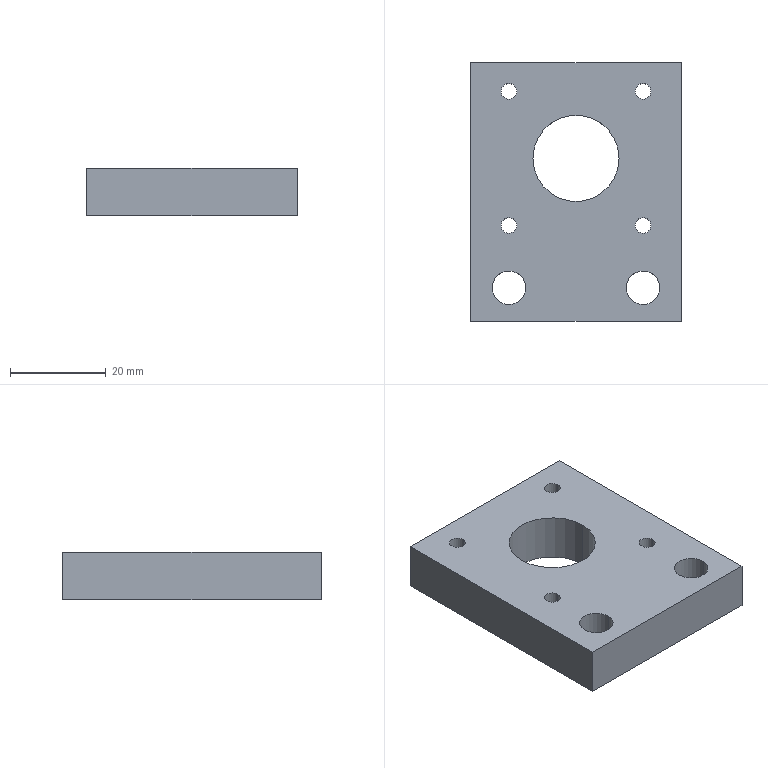Part | NX | 1 solid | 28 faces | box 44 x 54 x 10 mm | volume 20097 mm3 | cylinder 14 | cone 8 | plane 6 | commonest cylinder face diameters 3.3 x8 7 x4 18 x2
STEP:
#1=CARTESIAN_POINT('',(566.5,55.4,-338.82));
#2=VERTEX_POINT('',#1);
#3=CARTESIAN_POINT('',(573.5,55.4,-338.82));
#4=VERTEX_POINT('',#3);
#5=CARTESIAN_POINT('',(570.,55.4,-338.82));
#6=DIRECTION('',(0.,0.,1.));
#7=DIRECTION('',(1.,0.,0.));
#8=AXIS2_PLACEMENT_3D('',#5,#6,#7);
#9=CIRCLE('',#8,3.5);
#10=EDGE_CURVE('',#2,#4,#9,.T.);
#11=ORIENTED_EDGE('',*,*,#10,.F.);
#12=CARTESIAN_POINT('',(566.5,55.4,-328.82));
#13=VERTEX_POINT('',#12);
#14=CARTESIAN_POINT('',(566.5,55.4,-338.82));
#15=DIRECTION('',(0.,0.,1.));
#16=VECTOR('',#15,1000.);
#17=LINE('',#14,#16);
#18=EDGE_CURVE('',#2,#13,#17,.T.);
#19=ORIENTED_EDGE('',*,*,#18,.T.);
#20=CARTESIAN_POINT('',(573.5,55.4,-328.82));
#21=VERTEX_POINT('',#20);
#22=CARTESIAN_POINT('',(570.,55.4,-328.82));
#23=DIRECTION('',(0.,0.,1.));
#24=DIRECTION('',(1.,0.,0.));
#25=AXIS2_PLACEMENT_3D('',#22,#23,#24);
#26=CIRCLE('',#25,3.5);
#27=EDGE_CURVE('',#13,#21,#26,.T.);
#28=ORIENTED_EDGE('',*,*,#27,.T.);
#29=CARTESIAN_POINT('',(573.5,55.4,-338.82));
#30=DIRECTION('',(0.,0.,1.));
#31=VECTOR('',#30,1000.);
#32=LINE('',#29,#31);
#33=EDGE_CURVE('',#4,#21,#32,.T.);
#34=ORIENTED_EDGE('',*,*,#33,.F.);
#35=EDGE_LOOP('',(#11,#19,#28,#34));
#36=FACE_BOUND('',#35,.T.);
#37=CARTESIAN_POINT('',(570.,55.4,-338.82));
#38=DIRECTION('',(0.,0.,1.));
#39=DIRECTION('',(1.,0.,0.));
#40=AXIS2_PLACEMENT_3D('',#37,#38,#39);
#41=CYLINDRICAL_SURFACE('',#40,3.5);
#42=ADVANCED_FACE('',(#36),#41,.F.);
#43=CARTESIAN_POINT('',(578.,102.4,-338.82));
#44=VERTEX_POINT('',#43);
#45=CARTESIAN_POINT('',(578.,48.4,-338.82));
#46=VERTEX_POINT('',#45);
#47=CARTESIAN_POINT('',(578.,0.,-338.82));
#48=DIRECTION('',(0.,-1.,0.));
#49=VECTOR('',#48,1000.);
#50=LINE('',#47,#49);
#51=EDGE_CURVE('',#44,#46,#50,.T.);
#52=ORIENTED_EDGE('',*,*,#51,.F.);
#53=CARTESIAN_POINT('',(578.,102.4,-328.82));
#54=VERTEX_POINT('',#53);
#55=CARTESIAN_POINT('',(578.,102.4,-338.82));
#56=DIRECTION('',(0.,0.,1.));
#57=VECTOR('',#56,1000.);
#58=LINE('',#55,#57);
#59=EDGE_CURVE('',#44,#54,#58,.T.);
#60=ORIENTED_EDGE('',*,*,#59,.T.);
#61=CARTESIAN_POINT('',(578.,48.4,-328.82));
#62=VERTEX_POINT('',#61);
#63=CARTESIAN_POINT('',(578.,0.,-328.82));
#64=DIRECTION('',(0.,-1.,0.));
#65=VECTOR('',#64,1000.);
#66=LINE('',#63,#65);
#67=EDGE_CURVE('',#54,#62,#66,.T.);
#68=ORIENTED_EDGE('',*,*,#67,.T.);
#69=CARTESIAN_POINT('',(578.,48.4,-338.82));
#70=DIRECTION('',(0.,0.,1.));
#71=VECTOR('',#70,1000.);
#72=LINE('',#69,#71);
#73=EDGE_CURVE('',#46,#62,#72,.T.);
#74=ORIENTED_EDGE('',*,*,#73,.F.);
#75=EDGE_LOOP('',(#52,#60,#68,#74));
#76=FACE_BOUND('',#75,.T.);
#77=CARTESIAN_POINT('',(578.,102.4,-338.82));
#78=DIRECTION('',(1.,0.,0.));
#79=DIRECTION('',(0.,1.,0.));
#80=AXIS2_PLACEMENT_3D('',#77,#78,#79);
#81=PLANE('',#80);
#82=ADVANCED_FACE('',(#76),#81,.T.);
#83=CARTESIAN_POINT('',(534.,48.4,-338.82));
#84=VERTEX_POINT('',#83);
#85=CARTESIAN_POINT('',(0.,48.4,-338.82));
#86=DIRECTION('',(-1.,0.,0.));
#87=VECTOR('',#86,1000.);
#88=LINE('',#85,#87);
#89=EDGE_CURVE('',#46,#84,#88,.T.);
#90=ORIENTED_EDGE('',*,*,#89,.F.);
#91=ORIENTED_EDGE('',*,*,#73,.T.);
#92=CARTESIAN_POINT('',(534.,48.4,-328.82));
#93=VERTEX_POINT('',#92);
#94=CARTESIAN_POINT('',(0.,48.4,-328.82));
#95=DIRECTION('',(-1.,0.,0.));
#96=VECTOR('',#95,1000.);
#97=LINE('',#94,#96);
#98=EDGE_CURVE('',#62,#93,#97,.T.);
#99=ORIENTED_EDGE('',*,*,#98,.T.);
#100=CARTESIAN_POINT('',(534.,48.4,-338.82));
#101=DIRECTION('',(0.,0.,1.));
#102=VECTOR('',#101,1000.);
#103=LINE('',#100,#102);
#104=EDGE_CURVE('',#84,#93,#103,.T.);
#105=ORIENTED_EDGE('',*,*,#104,.F.);
#106=EDGE_LOOP('',(#90,#91,#99,#105));
#107=FACE_BOUND('',#106,.T.);
#108=CARTESIAN_POINT('',(578.,48.4,-338.82));
#109=DIRECTION('',(0.,-1.,0.));
#110=DIRECTION('',(0.,0.,-1.));
#111=AXIS2_PLACEMENT_3D('',#108,#109,#110);
#112=PLANE('',#111);
#113=ADVANCED_FACE('',(#107),#112,.T.);
#114=CARTESIAN_POINT('',(534.,102.4,-338.82));
#115=VERTEX_POINT('',#114);
#116=CARTESIAN_POINT('',(0.,102.4,-338.82));
#117=DIRECTION('',(1.,0.,0.));
#118=VECTOR('',#117,1000.);
#119=LINE('',#116,#118);
#120=EDGE_CURVE('',#115,#44,#119,.T.);
#121=ORIENTED_EDGE('',*,*,#120,.F.);
#122=CARTESIAN_POINT('',(534.,102.4,-328.82));
#123=VERTEX_POINT('',#122);
#124=CARTESIAN_POINT('',(534.,102.4,-338.82));
#125=DIRECTION('',(0.,0.,1.));
#126=VECTOR('',#125,1000.);
#127=LINE('',#124,#126);
#128=EDGE_CURVE('',#115,#123,#127,.T.);
#129=ORIENTED_EDGE('',*,*,#128,.T.);
#130=CARTESIAN_POINT('',(0.,102.4,-328.82));
#131=DIRECTION('',(1.,0.,0.));
#132=VECTOR('',#131,1000.);
#133=LINE('',#130,#132);
#134=EDGE_CURVE('',#123,#54,#133,.T.);
#135=ORIENTED_EDGE('',*,*,#134,.T.);
#136=ORIENTED_EDGE('',*,*,#59,.F.);
#137=EDGE_LOOP('',(#121,#129,#135,#136));
#138=FACE_BOUND('',#137,.T.);
#139=CARTESIAN_POINT('',(534.,102.4,-338.82));
#140=DIRECTION('',(0.,1.,0.));
#141=DIRECTION('',(1.,0.,0.));
#142=AXIS2_PLACEMENT_3D('',#139,#140,#141);
#143=PLANE('',#142);
#144=ADVANCED_FACE('',(#138),#143,.T.);
#145=ORIENTED_EDGE('',*,*,#134,.F.);
#146=CARTESIAN_POINT('',(534.,0.,-328.82));
#147=DIRECTION('',(0.,1.,0.));
#148=VECTOR('',#147,1000.);
#149=LINE('',#146,#148);
#150=EDGE_CURVE('',#93,#123,#149,.T.);
#151=ORIENTED_EDGE('',*,*,#150,.F.);
#152=ORIENTED_EDGE('',*,*,#98,.F.);
#153=ORIENTED_EDGE('',*,*,#67,.F.);
#154=EDGE_LOOP('',(#145,#151,#152,#153));
#155=FACE_BOUND('',#154,.T.);
#156=CARTESIAN_POINT('',(545.5,55.4,-328.82));
#157=VERTEX_POINT('',#156);
#158=CARTESIAN_POINT('',(538.5,55.4,-328.82));
#159=VERTEX_POINT('',#158);
#160=CARTESIAN_POINT('',(542.,55.4,-328.82));
#161=DIRECTION('',(0.,0.,1.));
#162=DIRECTION('',(1.,0.,0.));
#163=AXIS2_PLACEMENT_3D('',#160,#161,#162);
#164=CIRCLE('',#163,3.5);
#165=EDGE_CURVE('',#157,#159,#164,.T.);
#166=ORIENTED_EDGE('',*,*,#165,.F.);
#167=CARTESIAN_POINT('',(542.,55.4,-328.82));
#168=DIRECTION('',(0.,0.,1.));
#169=DIRECTION('',(1.,0.,0.));
#170=AXIS2_PLACEMENT_3D('',#167,#168,#169);
#171=CIRCLE('',#170,3.5);
#172=EDGE_CURVE('',#159,#157,#171,.T.);
#173=ORIENTED_EDGE('',*,*,#172,.F.);
#174=EDGE_LOOP('',(#166,#173));
#175=FACE_BOUND('',#174,.T.);
#176=ORIENTED_EDGE('',*,*,#27,.F.);
#177=CARTESIAN_POINT('',(570.,55.4,-328.82));
#178=DIRECTION('',(0.,0.,1.));
#179=DIRECTION('',(1.,0.,0.));
#180=AXIS2_PLACEMENT_3D('',#177,#178,#179);
#181=CIRCLE('',#180,3.5);
#182=EDGE_CURVE('',#21,#13,#181,.T.);
#183=ORIENTED_EDGE('',*,*,#182,.F.);
#184=EDGE_LOOP('',(#176,#183));
#185=FACE_BOUND('',#184,.T.);
#186=CARTESIAN_POINT('',(547.,82.4,-328.82));
#187=VERTEX_POINT('',#186);
#188=CARTESIAN_POINT('',(565.,82.4,-328.82));
#189=VERTEX_POINT('',#188);
#190=CARTESIAN_POINT('',(556.,82.4,-328.82));
#191=DIRECTION('',(0.,0.,1.));
#192=DIRECTION('',(1.,0.,0.));
#193=AXIS2_PLACEMENT_3D('',#190,#191,#192);
#194=CIRCLE('',#193,9.);
#195=EDGE_CURVE('',#187,#189,#194,.T.);
#196=ORIENTED_EDGE('',*,*,#195,.F.);
#197=CARTESIAN_POINT('',(556.,82.4,-328.82));
#198=DIRECTION('',(0.,0.,1.));
#199=DIRECTION('',(1.,0.,0.));
#200=AXIS2_PLACEMENT_3D('',#197,#198,#199);
#201=CIRCLE('',#200,9.);
#202=EDGE_CURVE('',#189,#187,#201,.T.);
#203=ORIENTED_EDGE('',*,*,#202,.F.);
#204=EDGE_LOOP('',(#196,#203));
#205=FACE_BOUND('',#204,.T.);
#206=CARTESIAN_POINT('',(540.35,96.4,-328.82));
#207=VERTEX_POINT('',#206);
#208=CARTESIAN_POINT('',(543.65,96.4,-328.82));
#209=VERTEX_POINT('',#208);
#210=CARTESIAN_POINT('',(542.,96.4,-328.82));
#211=DIRECTION('',(0.,0.,-1.));
#212=DIRECTION('',(-1.,0.,0.));
#213=AXIS2_PLACEMENT_3D('',#210,#211,#212);
#214=CIRCLE('',#213,1.65);
#215=EDGE_CURVE('',#207,#209,#214,.T.);
#216=ORIENTED_EDGE('',*,*,#215,.T.);
#217=CARTESIAN_POINT('',(542.,96.4,-328.82));
#218=DIRECTION('',(0.,0.,-1.));
#219=DIRECTION('',(-1.,0.,0.));
#220=AXIS2_PLACEMENT_3D('',#217,#218,#219);
#221=CIRCLE('',#220,1.65);
#222=EDGE_CURVE('',#209,#207,#221,.T.);
#223=ORIENTED_EDGE('',*,*,#222,.T.);
#224=EDGE_LOOP('',(#216,#223));
#225=FACE_BOUND('',#224,.T.);
#226=CARTESIAN_POINT('',(540.35,68.4,-328.82));
#227=VERTEX_POINT('',#226);
#228=CARTESIAN_POINT('',(543.65,68.4,-328.82));
#229=VERTEX_POINT('',#228);
#230=CARTESIAN_POINT('',(542.,68.4,-328.82));
#231=DIRECTION('',(0.,0.,-1.));
#232=DIRECTION('',(-1.,0.,0.));
#233=AXIS2_PLACEMENT_3D('',#230,#231,#232);
#234=CIRCLE('',#233,1.65);
#235=EDGE_CURVE('',#227,#229,#234,.T.);
#236=ORIENTED_EDGE('',*,*,#235,.T.);
#237=CARTESIAN_POINT('',(542.,68.4,-328.82));
#238=DIRECTION('',(0.,0.,-1.));
#239=DIRECTION('',(-1.,0.,0.));
#240=AXIS2_PLACEMENT_3D('',#237,#238,#239);
#241=CIRCLE('',#240,1.65);
#242=EDGE_CURVE('',#229,#227,#241,.T.);
#243=ORIENTED_EDGE('',*,*,#242,.T.);
#244=EDGE_LOOP('',(#236,#243));
#245=FACE_BOUND('',#244,.T.);
#246=CARTESIAN_POINT('',(571.65,68.4,-328.82));
#247=VERTEX_POINT('',#246);
#248=CARTESIAN_POINT('',(568.35,68.4,-328.82));
#249=VERTEX_POINT('',#248);
#250=CARTESIAN_POINT('',(570.,68.4,-328.82));
#251=DIRECTION('',(0.,0.,-1.));
#252=DIRECTION('',(-1.,0.,0.));
#253=AXIS2_PLACEMENT_3D('',#250,#251,#252);
#254=CIRCLE('',#253,1.65);
#255=EDGE_CURVE('',#247,#249,#254,.T.);
#256=ORIENTED_EDGE('',*,*,#255,.T.);
#257=CARTESIAN_POINT('',(570.,68.4,-328.82));
#258=DIRECTION('',(0.,0.,-1.));
#259=DIRECTION('',(-1.,0.,0.));
#260=AXIS2_PLACEMENT_3D('',#257,#258,#259);
#261=CIRCLE('',#260,1.65);
#262=EDGE_CURVE('',#249,#247,#261,.T.);
#263=ORIENTED_EDGE('',*,*,#262,.T.);
#264=EDGE_LOOP('',(#256,#263));
#265=FACE_BOUND('',#264,.T.);
#266=CARTESIAN_POINT('',(568.35,96.4,-328.82));
#267=VERTEX_POINT('',#266);
#268=CARTESIAN_POINT('',(571.65,96.4,-328.82));
#269=VERTEX_POINT('',#268);
#270=CARTESIAN_POINT('',(570.,96.4,-328.82));
#271=DIRECTION('',(0.,0.,-1.));
#272=DIRECTION('',(-1.,0.,0.));
#273=AXIS2_PLACEMENT_3D('',#270,#271,#272);
#274=CIRCLE('',#273,1.65);
#275=EDGE_CURVE('',#267,#269,#274,.T.);
#276=ORIENTED_EDGE('',*,*,#275,.T.);
#277=CARTESIAN_POINT('',(570.,96.4,-328.82));
#278=DIRECTION('',(0.,0.,-1.));
#279=DIRECTION('',(-1.,0.,0.));
#280=AXIS2_PLACEMENT_3D('',#277,#278,#279);
#281=CIRCLE('',#280,1.65);
#282=EDGE_CURVE('',#269,#267,#281,.T.);
#283=ORIENTED_EDGE('',*,*,#282,.T.);
#284=EDGE_LOOP('',(#276,#283));
#285=FACE_BOUND('',#284,.T.);
#286=CARTESIAN_POINT('',(565.967,77.363,-328.82));
#287=DIRECTION('',(0.,0.,1.));
#288=DIRECTION('',(1.,0.,0.));
#289=AXIS2_PLACEMENT_3D('',#286,#287,#288);
#290=PLANE('',#289);
#291=ADVANCED_FACE('',(#155,#175,#185,#205,#225,#245,#265,#285),#290,.T.);
#292=ORIENTED_EDGE('',*,*,#195,.T.);
#293=CARTESIAN_POINT('',(565.,82.4,-338.82));
#294=VERTEX_POINT('',#293);
#295=CARTESIAN_POINT('',(565.,82.4,-339.82));
#296=DIRECTION('',(0.,0.,1.));
#297=VECTOR('',#296,1000.);
#298=LINE('',#295,#297);
#299=EDGE_CURVE('',#294,#189,#298,.T.);
#300=ORIENTED_EDGE('',*,*,#299,.F.);
#301=CARTESIAN_POINT('',(547.,82.4,-338.82));
#302=VERTEX_POINT('',#301);
#303=CARTESIAN_POINT('',(556.,82.4,-338.82));
#304=DIRECTION('',(0.,0.,1.));
#305=DIRECTION('',(1.,0.,0.));
#306=AXIS2_PLACEMENT_3D('',#303,#304,#305);
#307=CIRCLE('',#306,9.);
#308=EDGE_CURVE('',#302,#294,#307,.T.);
#309=ORIENTED_EDGE('',*,*,#308,.F.);
#310=CARTESIAN_POINT('',(547.,82.4,-339.82));
#311=DIRECTION('',(0.,0.,1.));
#312=VECTOR('',#311,1000.);
#313=LINE('',#310,#312);
#314=EDGE_CURVE('',#302,#187,#313,.T.);
#315=ORIENTED_EDGE('',*,*,#314,.T.);
#316=EDGE_LOOP('',(#292,#300,#309,#315));
#317=FACE_BOUND('',#316,.T.);
#318=CARTESIAN_POINT('',(556.,82.4,-339.82));
#319=DIRECTION('',(0.,0.,1.));
#320=DIRECTION('',(1.,0.,0.));
#321=AXIS2_PLACEMENT_3D('',#318,#319,#320);
#322=CYLINDRICAL_SURFACE('',#321,9.);
#323=ADVANCED_FACE('',(#317),#322,.F.);
#324=CARTESIAN_POINT('',(534.,0.,-338.82));
#325=DIRECTION('',(0.,1.,0.));
#326=VECTOR('',#325,1000.);
#327=LINE('',#324,#326);
#328=EDGE_CURVE('',#84,#115,#327,.T.);
#329=ORIENTED_EDGE('',*,*,#328,.F.);
#330=ORIENTED_EDGE('',*,*,#104,.T.);
#331=ORIENTED_EDGE('',*,*,#150,.T.);
#332=ORIENTED_EDGE('',*,*,#128,.F.);
#333=EDGE_LOOP('',(#329,#330,#331,#332));
#334=FACE_BOUND('',#333,.T.);
#335=CARTESIAN_POINT('',(534.,48.4,-338.82));
#336=DIRECTION('',(-1.,0.,0.));
#337=DIRECTION('',(0.,0.,1.));
#338=AXIS2_PLACEMENT_3D('',#335,#336,#337);
#339=PLANE('',#338);
#340=ADVANCED_FACE('',(#334),#339,.T.);
#341=CARTESIAN_POINT('',(545.5,55.4,-338.82));
#342=VERTEX_POINT('',#341);
#343=CARTESIAN_POINT('',(538.5,55.4,-338.82));
#344=VERTEX_POINT('',#343);
#345=CARTESIAN_POINT('',(542.,55.4,-338.82));
#346=DIRECTION('',(0.,0.,1.));
#347=DIRECTION('',(1.,0.,0.));
#348=AXIS2_PLACEMENT_3D('',#345,#346,#347);
#349=CIRCLE('',#348,3.5);
#350=EDGE_CURVE('',#342,#344,#349,.T.);
#351=ORIENTED_EDGE('',*,*,#350,.F.);
#352=CARTESIAN_POINT('',(545.5,55.4,-338.82));
#353=DIRECTION('',(0.,0.,1.));
#354=VECTOR('',#353,1000.);
#355=LINE('',#352,#354);
#356=EDGE_CURVE('',#342,#157,#355,.T.);
#357=ORIENTED_EDGE('',*,*,#356,.T.);
#358=ORIENTED_EDGE('',*,*,#165,.T.);
#359=CARTESIAN_POINT('',(538.5,55.4,-338.82));
#360=DIRECTION('',(0.,0.,1.));
#361=VECTOR('',#360,1000.);
#362=LINE('',#359,#361);
#363=EDGE_CURVE('',#344,#159,#362,.T.);
#364=ORIENTED_EDGE('',*,*,#363,.F.);
#365=EDGE_LOOP('',(#351,#357,#358,#364));
#366=FACE_BOUND('',#365,.T.);
#367=CARTESIAN_POINT('',(542.,55.4,-338.82));
#368=DIRECTION('',(0.,0.,1.));
#369=DIRECTION('',(1.,0.,0.));
#370=AXIS2_PLACEMENT_3D('',#367,#368,#369);
#371=CYLINDRICAL_SURFACE('',#370,3.5);
#372=ADVANCED_FACE('',(#366),#371,.F.);
#373=ORIENTED_EDGE('',*,*,#51,.T.);
#374=ORIENTED_EDGE('',*,*,#89,.T.);
#375=ORIENTED_EDGE('',*,*,#328,.T.);
#376=ORIENTED_EDGE('',*,*,#120,.T.);
#377=EDGE_LOOP('',(#373,#374,#375,#376));
#378=FACE_BOUND('',#377,.T.);
#379=ORIENTED_EDGE('',*,*,#350,.T.);
#380=CARTESIAN_POINT('',(542.,55.4,-338.82));
#381=DIRECTION('',(0.,0.,1.));
#382=DIRECTION('',(1.,0.,0.));
#383=AXIS2_PLACEMENT_3D('',#380,#381,#382);
#384=CIRCLE('',#383,3.5);
#385=EDGE_CURVE('',#344,#342,#384,.T.);
#386=ORIENTED_EDGE('',*,*,#385,.T.);
#387=EDGE_LOOP('',(#379,#386));
#388=FACE_BOUND('',#387,.T.);
#389=CARTESIAN_POINT('',(572.315,96.4,-338.82));
#390=VERTEX_POINT('',#389);
#391=CARTESIAN_POINT('',(567.685,96.4,-338.82));
#392=VERTEX_POINT('',#391);
#393=CARTESIAN_POINT('',(570.,96.4,-338.82));
#394=DIRECTION('',(0.,0.,-1.));
#395=DIRECTION('',(-1.,0.,0.));
#396=AXIS2_PLACEMENT_3D('',#393,#394,#395);
#397=CIRCLE('',#396,2.315);
#398=EDGE_CURVE('',#390,#392,#397,.T.);
#399=ORIENTED_EDGE('',*,*,#398,.F.);
#400=CARTESIAN_POINT('',(570.,96.4,-338.82));
#401=DIRECTION('',(0.,0.,-1.));
#402=DIRECTION('',(-1.,0.,0.));
#403=AXIS2_PLACEMENT_3D('',#400,#401,#402);
#404=CIRCLE('',#403,2.315);
#405=EDGE_CURVE('',#392,#390,#404,.T.);
#406=ORIENTED_EDGE('',*,*,#405,.F.);
#407=EDGE_LOOP('',(#399,#406));
#408=FACE_BOUND('',#407,.T.);
#409=CARTESIAN_POINT('',(544.315,68.4,-338.82));
#410=VERTEX_POINT('',#409);
#411=CARTESIAN_POINT('',(539.685,68.4,-338.82));
#412=VERTEX_POINT('',#411);
#413=CARTESIAN_POINT('',(542.,68.4,-338.82));
#414=DIRECTION('',(0.,0.,-1.));
#415=DIRECTION('',(-1.,0.,0.));
#416=AXIS2_PLACEMENT_3D('',#413,#414,#415);
#417=CIRCLE('',#416,2.315);
#418=EDGE_CURVE('',#410,#412,#417,.T.);
#419=ORIENTED_EDGE('',*,*,#418,.F.);
#420=CARTESIAN_POINT('',(542.,68.4,-338.82));
#421=DIRECTION('',(0.,0.,-1.));
#422=DIRECTION('',(-1.,0.,0.));
#423=AXIS2_PLACEMENT_3D('',#420,#421,#422);
#424=CIRCLE('',#423,2.315);
#425=EDGE_CURVE('',#412,#410,#424,.T.);
#426=ORIENTED_EDGE('',*,*,#425,.F.);
#427=EDGE_LOOP('',(#419,#426));
#428=FACE_BOUND('',#427,.T.);
#429=ORIENTED_EDGE('',*,*,#10,.T.);
#430=CARTESIAN_POINT('',(570.,55.4,-338.82));
#431=DIRECTION('',(0.,0.,1.));
#432=DIRECTION('',(1.,0.,0.));
#433=AXIS2_PLACEMENT_3D('',#430,#431,#432);
#434=CIRCLE('',#433,3.5);
#435=EDGE_CURVE('',#4,#2,#434,.T.);
#436=ORIENTED_EDGE('',*,*,#435,.T.);
#437=EDGE_LOOP('',(#429,#436));
#438=FACE_BOUND('',#437,.T.);
#439=CARTESIAN_POINT('',(556.,82.4,-338.82));
#440=DIRECTION('',(0.,0.,1.));
#441=DIRECTION('',(1.,0.,0.));
#442=AXIS2_PLACEMENT_3D('',#439,#440,#441);
#443=CIRCLE('',#442,9.);
#444=EDGE_CURVE('',#294,#302,#443,.T.);
#445=ORIENTED_EDGE('',*,*,#444,.T.);
#446=ORIENTED_EDGE('',*,*,#308,.T.);
#447=EDGE_LOOP('',(#445,#446));
#448=FACE_BOUND('',#447,.T.);
#449=CARTESIAN_POINT('',(539.685,96.4,-338.82));
#450=VERTEX_POINT('',#449);
#451=CARTESIAN_POINT('',(544.315,96.4,-338.82));
#452=VERTEX_POINT('',#451);
#453=CARTESIAN_POINT('',(542.,96.4,-338.82));
#454=DIRECTION('',(0.,0.,-1.));
#455=DIRECTION('',(-1.,0.,0.));
#456=AXIS2_PLACEMENT_3D('',#453,#454,#455);
#457=CIRCLE('',#456,2.315);
#458=EDGE_CURVE('',#450,#452,#457,.T.);
#459=ORIENTED_EDGE('',*,*,#458,.F.);
#460=CARTESIAN_POINT('',(542.,96.4,-338.82));
#461=DIRECTION('',(0.,0.,-1.));
#462=DIRECTION('',(-1.,0.,0.));
#463=AXIS2_PLACEMENT_3D('',#460,#461,#462);
#464=CIRCLE('',#463,2.315);
#465=EDGE_CURVE('',#452,#450,#464,.T.);
#466=ORIENTED_EDGE('',*,*,#465,.F.);
#467=EDGE_LOOP('',(#459,#466));
#468=FACE_BOUND('',#467,.T.);
#469=CARTESIAN_POINT('',(567.685,68.4,-338.82));
#470=VERTEX_POINT('',#469);
#471=CARTESIAN_POINT('',(572.315,68.4,-338.82));
#472=VERTEX_POINT('',#471);
#473=CARTESIAN_POINT('',(570.,68.4,-338.82));
#474=DIRECTION('',(0.,0.,-1.));
#475=DIRECTION('',(-1.,0.,0.));
#476=AXIS2_PLACEMENT_3D('',#473,#474,#475);
#477=CIRCLE('',#476,2.315);
#478=EDGE_CURVE('',#470,#472,#477,.T.);
#479=ORIENTED_EDGE('',*,*,#478,.F.);
#480=CARTESIAN_POINT('',(570.,68.4,-338.82));
#481=DIRECTION('',(0.,0.,-1.));
#482=DIRECTION('',(-1.,0.,0.));
#483=AXIS2_PLACEMENT_3D('',#480,#481,#482);
#484=CIRCLE('',#483,2.315);
#485=EDGE_CURVE('',#472,#470,#484,.T.);
#486=ORIENTED_EDGE('',*,*,#485,.F.);
#487=EDGE_LOOP('',(#479,#486));
#488=FACE_BOUND('',#487,.T.);
#489=CARTESIAN_POINT('',(565.967,77.363,-338.82));
#490=DIRECTION('',(0.,0.,1.));
#491=DIRECTION('',(1.,0.,0.));
#492=AXIS2_PLACEMENT_3D('',#489,#490,#491);
#493=PLANE('',#492);
#494=ADVANCED_FACE('',(#378,#388,#408,#428,#438,#448,#468,#488),#493,.F.);
#495=ORIENTED_EDGE('',*,*,#215,.F.);
#496=CARTESIAN_POINT('',(540.35,96.4,-338.436));
#497=VERTEX_POINT('',#496);
#498=CARTESIAN_POINT('',(540.35,96.4,-338.82));
#499=DIRECTION('',(0.,0.,-1.));
#500=VECTOR('',#499,1000.);
#501=LINE('',#498,#500);
#502=EDGE_CURVE('',#497,#207,#501,.F.);
#503=ORIENTED_EDGE('',*,*,#502,.F.);
#504=CARTESIAN_POINT('',(543.65,96.4,-338.436));
#505=VERTEX_POINT('',#504);
#506=CARTESIAN_POINT('',(542.,96.4,-338.436));
#507=DIRECTION('',(0.,0.,-1.));
#508=DIRECTION('',(-1.,0.,0.));
#509=AXIS2_PLACEMENT_3D('',#506,#507,#508);
#510=CIRCLE('',#509,1.65);
#511=EDGE_CURVE('',#497,#505,#510,.T.);
#512=ORIENTED_EDGE('',*,*,#511,.T.);
#513=CARTESIAN_POINT('',(543.65,96.4,-338.82));
#514=DIRECTION('',(0.,0.,-1.));
#515=VECTOR('',#514,1000.);
#516=LINE('',#513,#515);
#517=EDGE_CURVE('',#505,#209,#516,.F.);
#518=ORIENTED_EDGE('',*,*,#517,.T.);
#519=EDGE_LOOP('',(#495,#503,#512,#518));
#520=FACE_BOUND('',#519,.T.);
#521=CARTESIAN_POINT('',(542.,96.4,-338.82));
#522=DIRECTION('',(0.,0.,-1.));
#523=DIRECTION('',(-1.,0.,0.));
#524=AXIS2_PLACEMENT_3D('',#521,#522,#523);
#525=CYLINDRICAL_SURFACE('',#524,1.65);
#526=ADVANCED_FACE('',(#520),#525,.F.);
#527=CARTESIAN_POINT('',(542.,96.4,-338.436));
#528=DIRECTION('',(0.,0.,-1.));
#529=DIRECTION('',(-1.,0.,0.));
#530=AXIS2_PLACEMENT_3D('',#527,#528,#529);
#531=CIRCLE('',#530,1.65);
#532=EDGE_CURVE('',#505,#497,#531,.T.);
#533=ORIENTED_EDGE('',*,*,#532,.F.);
#534=CARTESIAN_POINT('',(543.65,96.4,-338.436));
#535=DIRECTION('',(0.866,0.,-0.5));
#536=VECTOR('',#535,1000.);
#537=LINE('',#534,#536);
#538=EDGE_CURVE('',#505,#452,#537,.T.);
#539=ORIENTED_EDGE('',*,*,#538,.T.);
#540=ORIENTED_EDGE('',*,*,#465,.T.);
#541=CARTESIAN_POINT('',(540.35,96.4,-338.436));
#542=DIRECTION('',(-0.866,0.,-0.5));
#543=VECTOR('',#542,1000.);
#544=LINE('',#541,#543);
#545=EDGE_CURVE('',#497,#450,#544,.T.);
#546=ORIENTED_EDGE('',*,*,#545,.F.);
#547=EDGE_LOOP('',(#533,#539,#540,#546));
#548=FACE_BOUND('',#547,.T.);
#549=CARTESIAN_POINT('',(542.,96.4,-338.436));
#550=DIRECTION('',(0.,0.,-1.));
#551=DIRECTION('',(-1.,0.,0.));
#552=AXIS2_PLACEMENT_3D('',#549,#550,#551);
#553=CONICAL_SURFACE('',#552,1.65,1.047);
#554=ADVANCED_FACE('',(#548),#553,.F.);
#555=CARTESIAN_POINT('',(540.35,68.4,-338.436));
#556=VERTEX_POINT('',#555);
#557=CARTESIAN_POINT('',(543.65,68.4,-338.436));
#558=VERTEX_POINT('',#557);
#559=CARTESIAN_POINT('',(542.,68.4,-338.436));
#560=DIRECTION('',(0.,0.,-1.));
#561=DIRECTION('',(-1.,0.,0.));
#562=AXIS2_PLACEMENT_3D('',#559,#560,#561);
#563=CIRCLE('',#562,1.65);
#564=EDGE_CURVE('',#556,#558,#563,.T.);
#565=ORIENTED_EDGE('',*,*,#564,.T.);
#566=CARTESIAN_POINT('',(543.65,68.4,-338.82));
#567=DIRECTION('',(0.,0.,-1.));
#568=VECTOR('',#567,1000.);
#569=LINE('',#566,#568);
#570=EDGE_CURVE('',#558,#229,#569,.F.);
#571=ORIENTED_EDGE('',*,*,#570,.T.);
#572=ORIENTED_EDGE('',*,*,#235,.F.);
#573=CARTESIAN_POINT('',(540.35,68.4,-338.82));
#574=DIRECTION('',(0.,0.,-1.));
#575=VECTOR('',#574,1000.);
#576=LINE('',#573,#575);
#577=EDGE_CURVE('',#556,#227,#576,.F.);
#578=ORIENTED_EDGE('',*,*,#577,.F.);
#579=EDGE_LOOP('',(#565,#571,#572,#578));
#580=FACE_BOUND('',#579,.T.);
#581=CARTESIAN_POINT('',(542.,68.4,-338.82));
#582=DIRECTION('',(0.,0.,-1.));
#583=DIRECTION('',(-1.,0.,0.));
#584=AXIS2_PLACEMENT_3D('',#581,#582,#583);
#585=CYLINDRICAL_SURFACE('',#584,1.65);
#586=ADVANCED_FACE('',(#580),#585,.F.);
#587=ORIENTED_EDGE('',*,*,#564,.F.);
#588=CARTESIAN_POINT('',(540.35,68.4,-338.436));
#589=DIRECTION('',(-0.866,0.,-0.5));
#590=VECTOR('',#589,1000.);
#591=LINE('',#588,#590);
#592=EDGE_CURVE('',#412,#556,#591,.F.);
#593=ORIENTED_EDGE('',*,*,#592,.F.);
#594=ORIENTED_EDGE('',*,*,#425,.T.);
#595=CARTESIAN_POINT('',(543.65,68.4,-338.436));
#596=DIRECTION('',(0.866,0.,-0.5));
#597=VECTOR('',#596,1000.);
#598=LINE('',#595,#597);
#599=EDGE_CURVE('',#410,#558,#598,.F.);
#600=ORIENTED_EDGE('',*,*,#599,.T.);
#601=EDGE_LOOP('',(#587,#593,#594,#600));
#602=FACE_BOUND('',#601,.T.);
#603=CARTESIAN_POINT('',(542.,68.4,-338.436));
#604=DIRECTION('',(0.,0.,-1.));
#605=DIRECTION('',(-1.,0.,0.));
#606=AXIS2_PLACEMENT_3D('',#603,#604,#605);
#607=CONICAL_SURFACE('',#606,1.65,1.047);
#608=ADVANCED_FACE('',(#602),#607,.F.);
#609=ORIENTED_EDGE('',*,*,#255,.F.);
#610=CARTESIAN_POINT('',(571.65,68.4,-338.436));
#611=VERTEX_POINT('',#610);
#612=CARTESIAN_POINT('',(571.65,68.4,-338.82));
#613=DIRECTION('',(0.,0.,-1.));
#614=VECTOR('',#613,1000.);
#615=LINE('',#612,#614);
#616=EDGE_CURVE('',#611,#247,#615,.F.);
#617=ORIENTED_EDGE('',*,*,#616,.F.);
#618=CARTESIAN_POINT('',(568.35,68.4,-338.436));
#619=VERTEX_POINT('',#618);
#620=CARTESIAN_POINT('',(570.,68.4,-338.436));
#621=DIRECTION('',(0.,0.,-1.));
#622=DIRECTION('',(-1.,0.,0.));
#623=AXIS2_PLACEMENT_3D('',#620,#621,#622);
#624=CIRCLE('',#623,1.65);
#625=EDGE_CURVE('',#611,#619,#624,.T.);
#626=ORIENTED_EDGE('',*,*,#625,.T.);
#627=CARTESIAN_POINT('',(568.35,68.4,-338.82));
#628=DIRECTION('',(0.,0.,-1.));
#629=VECTOR('',#628,1000.);
#630=LINE('',#627,#629);
#631=EDGE_CURVE('',#619,#249,#630,.F.);
#632=ORIENTED_EDGE('',*,*,#631,.T.);
#633=EDGE_LOOP('',(#609,#617,#626,#632));
#634=FACE_BOUND('',#633,.T.);
#635=CARTESIAN_POINT('',(570.,68.4,-338.82));
#636=DIRECTION('',(0.,0.,-1.));
#637=DIRECTION('',(-1.,0.,0.));
#638=AXIS2_PLACEMENT_3D('',#635,#636,#637);
#639=CYLINDRICAL_SURFACE('',#638,1.65);
#640=ADVANCED_FACE('',(#634),#639,.F.);
#641=ORIENTED_EDGE('',*,*,#625,.F.);
#642=CARTESIAN_POINT('',(571.65,68.4,-338.436));
#643=DIRECTION('',(0.866,0.,-0.5));
#644=VECTOR('',#643,1000.);
#645=LINE('',#642,#644);
#646=EDGE_CURVE('',#611,#472,#645,.T.);
#647=ORIENTED_EDGE('',*,*,#646,.T.);
#648=ORIENTED_EDGE('',*,*,#485,.T.);
#649=CARTESIAN_POINT('',(568.35,68.4,-338.436));
#650=DIRECTION('',(-0.866,0.,-0.5));
#651=VECTOR('',#650,1000.);
#652=LINE('',#649,#651);
#653=EDGE_CURVE('',#619,#470,#652,.T.);
#654=ORIENTED_EDGE('',*,*,#653,.F.);
#655=EDGE_LOOP('',(#641,#647,#648,#654));
#656=FACE_BOUND('',#655,.T.);
#657=CARTESIAN_POINT('',(570.,68.4,-338.436));
#658=DIRECTION('',(0.,0.,-1.));
#659=DIRECTION('',(-1.,0.,0.));
#660=AXIS2_PLACEMENT_3D('',#657,#658,#659);
#661=CONICAL_SURFACE('',#660,1.65,1.047);
#662=ADVANCED_FACE('',(#656),#661,.F.);
#663=CARTESIAN_POINT('',(571.65,96.4,-338.436));
#664=VERTEX_POINT('',#663);
#665=CARTESIAN_POINT('',(568.35,96.4,-338.436));
#666=VERTEX_POINT('',#665);
#667=CARTESIAN_POINT('',(570.,96.4,-338.436));
#668=DIRECTION('',(0.,0.,-1.));
#669=DIRECTION('',(-1.,0.,0.));
#670=AXIS2_PLACEMENT_3D('',#667,#668,#669);
#671=CIRCLE('',#670,1.65);
#672=EDGE_CURVE('',#664,#666,#671,.T.);
#673=ORIENTED_EDGE('',*,*,#672,.T.);
#674=CARTESIAN_POINT('',(568.35,96.4,-338.82));
#675=DIRECTION('',(0.,0.,-1.));
#676=VECTOR('',#675,1000.);
#677=LINE('',#674,#676);
#678=EDGE_CURVE('',#666,#267,#677,.F.);
#679=ORIENTED_EDGE('',*,*,#678,.T.);
#680=ORIENTED_EDGE('',*,*,#282,.F.);
#681=CARTESIAN_POINT('',(571.65,96.4,-338.82));
#682=DIRECTION('',(0.,0.,-1.));
#683=VECTOR('',#682,1000.);
#684=LINE('',#681,#683);
#685=EDGE_CURVE('',#664,#269,#684,.F.);
#686=ORIENTED_EDGE('',*,*,#685,.F.);
#687=EDGE_LOOP('',(#673,#679,#680,#686));
#688=FACE_BOUND('',#687,.T.);
#689=CARTESIAN_POINT('',(570.,96.4,-338.82));
#690=DIRECTION('',(0.,0.,-1.));
#691=DIRECTION('',(-1.,0.,0.));
#692=AXIS2_PLACEMENT_3D('',#689,#690,#691);
#693=CYLINDRICAL_SURFACE('',#692,1.65);
#694=ADVANCED_FACE('',(#688),#693,.F.);
#695=ORIENTED_EDGE('',*,*,#672,.F.);
#696=CARTESIAN_POINT('',(571.65,96.4,-338.436));
#697=DIRECTION('',(0.866,0.,-0.5));
#698=VECTOR('',#697,1000.);
#699=LINE('',#696,#698);
#700=EDGE_CURVE('',#390,#664,#699,.F.);
#701=ORIENTED_EDGE('',*,*,#700,.F.);
#702=ORIENTED_EDGE('',*,*,#398,.T.);
#703=CARTESIAN_POINT('',(568.35,96.4,-338.436));
#704=DIRECTION('',(-0.866,0.,-0.5));
#705=VECTOR('',#704,1000.);
#706=LINE('',#703,#705);
#707=EDGE_CURVE('',#392,#666,#706,.F.);
#708=ORIENTED_EDGE('',*,*,#707,.T.);
#709=EDGE_LOOP('',(#695,#701,#702,#708));
#710=FACE_BOUND('',#709,.T.);
#711=CARTESIAN_POINT('',(570.,96.4,-338.436));
#712=DIRECTION('',(0.,0.,-1.));
#713=DIRECTION('',(-1.,0.,0.));
#714=AXIS2_PLACEMENT_3D('',#711,#712,#713);
#715=CONICAL_SURFACE('',#714,1.65,1.047);
#716=ADVANCED_FACE('',(#710),#715,.F.);
#717=ORIENTED_EDGE('',*,*,#33,.T.);
#718=ORIENTED_EDGE('',*,*,#182,.T.);
#719=ORIENTED_EDGE('',*,*,#18,.F.);
#720=ORIENTED_EDGE('',*,*,#435,.F.);
#721=EDGE_LOOP('',(#717,#718,#719,#720));
#722=FACE_BOUND('',#721,.T.);
#723=CARTESIAN_POINT('',(570.,55.4,-338.82));
#724=DIRECTION('',(0.,0.,1.));
#725=DIRECTION('',(1.,0.,0.));
#726=AXIS2_PLACEMENT_3D('',#723,#724,#725);
#727=CYLINDRICAL_SURFACE('',#726,3.5);
#728=ADVANCED_FACE('',(#722),#727,.F.);
#729=ORIENTED_EDGE('',*,*,#707,.F.);
#730=ORIENTED_EDGE('',*,*,#405,.T.);
#731=ORIENTED_EDGE('',*,*,#700,.T.);
#732=CARTESIAN_POINT('',(570.,96.4,-338.436));
#733=DIRECTION('',(0.,0.,-1.));
#734=DIRECTION('',(-1.,0.,0.));
#735=AXIS2_PLACEMENT_3D('',#732,#733,#734);
#736=CIRCLE('',#735,1.65);
#737=EDGE_CURVE('',#666,#664,#736,.T.);
#738=ORIENTED_EDGE('',*,*,#737,.F.);
#739=EDGE_LOOP('',(#729,#730,#731,#738));
#740=FACE_BOUND('',#739,.T.);
#741=CARTESIAN_POINT('',(570.,96.4,-338.436));
#742=DIRECTION('',(0.,0.,-1.));
#743=DIRECTION('',(-1.,0.,0.));
#744=AXIS2_PLACEMENT_3D('',#741,#742,#743);
#745=CONICAL_SURFACE('',#744,1.65,1.047);
#746=ADVANCED_FACE('',(#740),#745,.F.);
#747=ORIENTED_EDGE('',*,*,#631,.F.);
#748=CARTESIAN_POINT('',(570.,68.4,-338.436));
#749=DIRECTION('',(0.,0.,-1.));
#750=DIRECTION('',(-1.,0.,0.));
#751=AXIS2_PLACEMENT_3D('',#748,#749,#750);
#752=CIRCLE('',#751,1.65);
#753=EDGE_CURVE('',#619,#611,#752,.T.);
#754=ORIENTED_EDGE('',*,*,#753,.T.);
#755=ORIENTED_EDGE('',*,*,#616,.T.);
#756=ORIENTED_EDGE('',*,*,#262,.F.);
#757=EDGE_LOOP('',(#747,#754,#755,#756));
#758=FACE_BOUND('',#757,.T.);
#759=CARTESIAN_POINT('',(570.,68.4,-338.82));
#760=DIRECTION('',(0.,0.,-1.));
#761=DIRECTION('',(-1.,0.,0.));
#762=AXIS2_PLACEMENT_3D('',#759,#760,#761);
#763=CYLINDRICAL_SURFACE('',#762,1.65);
#764=ADVANCED_FACE('',(#758),#763,.F.);
#765=ORIENTED_EDGE('',*,*,#458,.T.);
#766=ORIENTED_EDGE('',*,*,#538,.F.);
#767=ORIENTED_EDGE('',*,*,#511,.F.);
#768=ORIENTED_EDGE('',*,*,#545,.T.);
#769=EDGE_LOOP('',(#765,#766,#767,#768));
#770=FACE_BOUND('',#769,.T.);
#771=CARTESIAN_POINT('',(542.,96.4,-338.436));
#772=DIRECTION('',(0.,0.,-1.));
#773=DIRECTION('',(-1.,0.,0.));
#774=AXIS2_PLACEMENT_3D('',#771,#772,#773);
#775=CONICAL_SURFACE('',#774,1.65,1.047);
#776=ADVANCED_FACE('',(#770),#775,.F.);
#777=ORIENTED_EDGE('',*,*,#356,.F.);
#778=ORIENTED_EDGE('',*,*,#385,.F.);
#779=ORIENTED_EDGE('',*,*,#363,.T.);
#780=ORIENTED_EDGE('',*,*,#172,.T.);
#781=EDGE_LOOP('',(#777,#778,#779,#780));
#782=FACE_BOUND('',#781,.T.);
#783=CARTESIAN_POINT('',(542.,55.4,-338.82));
#784=DIRECTION('',(0.,0.,1.));
#785=DIRECTION('',(1.,0.,0.));
#786=AXIS2_PLACEMENT_3D('',#783,#784,#785);
#787=CYLINDRICAL_SURFACE('',#786,3.5);
#788=ADVANCED_FACE('',(#782),#787,.F.);
#789=ORIENTED_EDGE('',*,*,#478,.T.);
#790=ORIENTED_EDGE('',*,*,#646,.F.);
#791=ORIENTED_EDGE('',*,*,#753,.F.);
#792=ORIENTED_EDGE('',*,*,#653,.T.);
#793=EDGE_LOOP('',(#789,#790,#791,#792));
#794=FACE_BOUND('',#793,.T.);
#795=CARTESIAN_POINT('',(570.,68.4,-338.436));
#796=DIRECTION('',(0.,0.,-1.));
#797=DIRECTION('',(-1.,0.,0.));
#798=AXIS2_PLACEMENT_3D('',#795,#796,#797);
#799=CONICAL_SURFACE('',#798,1.65,1.047);
#800=ADVANCED_FACE('',(#794),#799,.F.);
#801=ORIENTED_EDGE('',*,*,#577,.T.);
#802=ORIENTED_EDGE('',*,*,#242,.F.);
#803=ORIENTED_EDGE('',*,*,#570,.F.);
#804=CARTESIAN_POINT('',(542.,68.4,-338.436));
#805=DIRECTION('',(0.,0.,-1.));
#806=DIRECTION('',(-1.,0.,0.));
#807=AXIS2_PLACEMENT_3D('',#804,#805,#806);
#808=CIRCLE('',#807,1.65);
#809=EDGE_CURVE('',#558,#556,#808,.T.);
#810=ORIENTED_EDGE('',*,*,#809,.T.);
#811=EDGE_LOOP('',(#801,#802,#803,#810));
#812=FACE_BOUND('',#811,.T.);
#813=CARTESIAN_POINT('',(542.,68.4,-338.82));
#814=DIRECTION('',(0.,0.,-1.));
#815=DIRECTION('',(-1.,0.,0.));
#816=AXIS2_PLACEMENT_3D('',#813,#814,#815);
#817=CYLINDRICAL_SURFACE('',#816,1.65);
#818=ADVANCED_FACE('',(#812),#817,.F.);
#819=ORIENTED_EDGE('',*,*,#444,.F.);
#820=ORIENTED_EDGE('',*,*,#299,.T.);
#821=ORIENTED_EDGE('',*,*,#202,.T.);
#822=ORIENTED_EDGE('',*,*,#314,.F.);
#823=EDGE_LOOP('',(#819,#820,#821,#822));
#824=FACE_BOUND('',#823,.T.);
#825=CARTESIAN_POINT('',(556.,82.4,-339.82));
#826=DIRECTION('',(0.,0.,1.));
#827=DIRECTION('',(1.,0.,0.));
#828=AXIS2_PLACEMENT_3D('',#825,#826,#827);
#829=CYLINDRICAL_SURFACE('',#828,9.);
#830=ADVANCED_FACE('',(#824),#829,.F.);
#831=ORIENTED_EDGE('',*,*,#275,.F.);
#832=ORIENTED_EDGE('',*,*,#678,.F.);
#833=ORIENTED_EDGE('',*,*,#737,.T.);
#834=ORIENTED_EDGE('',*,*,#685,.T.);
#835=EDGE_LOOP('',(#831,#832,#833,#834));
#836=FACE_BOUND('',#835,.T.);
#837=CARTESIAN_POINT('',(570.,96.4,-338.82));
#838=DIRECTION('',(0.,0.,-1.));
#839=DIRECTION('',(-1.,0.,0.));
#840=AXIS2_PLACEMENT_3D('',#837,#838,#839);
#841=CYLINDRICAL_SURFACE('',#840,1.65);
#842=ADVANCED_FACE('',(#836),#841,.F.);
#843=ORIENTED_EDGE('',*,*,#418,.T.);
#844=ORIENTED_EDGE('',*,*,#592,.T.);
#845=ORIENTED_EDGE('',*,*,#809,.F.);
#846=ORIENTED_EDGE('',*,*,#599,.F.);
#847=EDGE_LOOP('',(#843,#844,#845,#846));
#848=FACE_BOUND('',#847,.T.);
#849=CARTESIAN_POINT('',(542.,68.4,-338.436));
#850=DIRECTION('',(0.,0.,-1.));
#851=DIRECTION('',(-1.,0.,0.));
#852=AXIS2_PLACEMENT_3D('',#849,#850,#851);
#853=CONICAL_SURFACE('',#852,1.65,1.047);
#854=ADVANCED_FACE('',(#848),#853,.F.);
#855=ORIENTED_EDGE('',*,*,#532,.T.);
#856=ORIENTED_EDGE('',*,*,#502,.T.);
#857=ORIENTED_EDGE('',*,*,#222,.F.);
#858=ORIENTED_EDGE('',*,*,#517,.F.);
#859=EDGE_LOOP('',(#855,#856,#857,#858));
#860=FACE_BOUND('',#859,.T.);
#861=CARTESIAN_POINT('',(542.,96.4,-338.82));
#862=DIRECTION('',(0.,0.,-1.));
#863=DIRECTION('',(-1.,0.,0.));
#864=AXIS2_PLACEMENT_3D('',#861,#862,#863);
#865=CYLINDRICAL_SURFACE('',#864,1.65);
#866=ADVANCED_FACE('',(#860),#865,.F.);
#867=CLOSED_SHELL('',(#42,#82,#113,#144,#291,#323,#340,#372,#494,#526,#554,#586,#608,#640,#662,#694,#716,#728,#746,#764,#776,#788,#800,#818,#830,#842,#854,#866));
#868=MANIFOLD_SOLID_BREP('',#867);
#869=(LENGTH_UNIT()NAMED_UNIT(*)SI_UNIT(.MILLI.,.METRE.));
#870=UNCERTAINTY_MEASURE_WITH_UNIT(LENGTH_MEASURE(0.00001),#869,'','');
#871=(NAMED_UNIT(*)PLANE_ANGLE_UNIT()SI_UNIT($,.RADIAN.));
#872=(NAMED_UNIT(*)SI_UNIT($,.STERADIAN.)SOLID_ANGLE_UNIT());
#873=(GEOMETRIC_REPRESENTATION_CONTEXT(3)GLOBAL_UNCERTAINTY_ASSIGNED_CONTEXT((#870))GLOBAL_UNIT_ASSIGNED_CONTEXT((#869,#871,#872))REPRESENTATION_CONTEXT('',''));
#874=ADVANCED_BREP_SHAPE_REPRESENTATION('',(#868),#873);